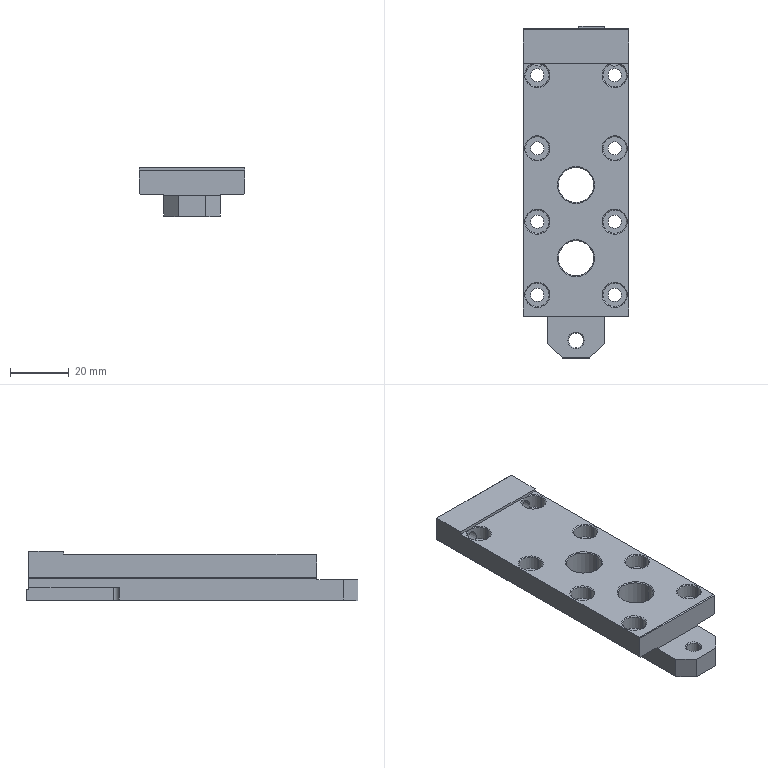Part | NX | 1 solid | 130 faces | box 36 x 113.3 x 17 mm | volume 37970 mm3 | cone 52 | cylinder 43 | plane 35 | commonest cylinder face diameters 4.5 x16 8 x16 5 x6 12 x4 4 x1